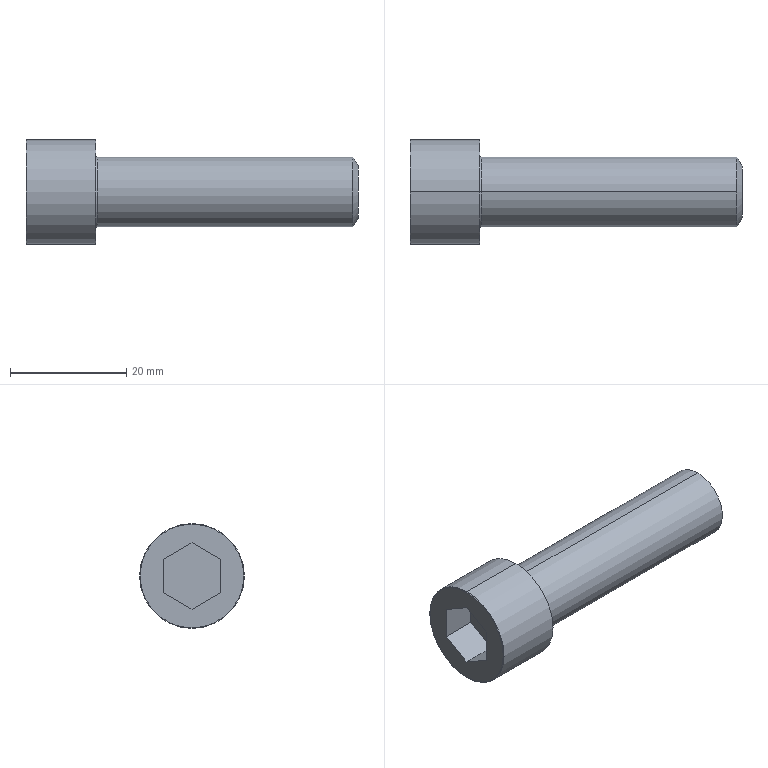Part | SolidWorks | features BlendCut 1, Cut 1, Fillet 1, LPattern 1, RevCut 1, Revolution 1 | 1 solid | 20 faces | box 57 x 18 x 18 mm | volume 7611 mm3 | plane 10 | torus 4 | cylinder 4 | cone 2 | commonest cylinder face diameters 12 x2 18 x2
STEP:
#1=CARTESIAN_POINT('',(0.,0.,8.9));
#2=VERTEX_POINT('',#1);
#3=CARTESIAN_POINT('',(0.,0.,-8.9));
#4=VERTEX_POINT('',#3);
#5=CARTESIAN_POINT('',(0.,0.,0.));
#6=DIRECTION('',(-1.,0.,0.));
#7=DIRECTION('',(0.,0.,-1.));
#8=AXIS2_PLACEMENT_3D('',#5,#6,#7);
#9=CIRCLE('',#8,8.9);
#10=EDGE_CURVE('',#2,#4,#9,.T.);
#11=ORIENTED_EDGE('',*,*,#10,.F.);
#12=CARTESIAN_POINT('',(0.1,0.,9.));
#13=VERTEX_POINT('',#12);
#14=CARTESIAN_POINT('',(0.1,0.,8.9));
#15=DIRECTION('',(0.,1.,0.));
#16=DIRECTION('',(0.,0.,1.));
#17=AXIS2_PLACEMENT_3D('',#14,#15,#16);
#18=CIRCLE('',#17,0.1);
#19=EDGE_CURVE('',#2,#13,#18,.T.);
#20=ORIENTED_EDGE('',*,*,#19,.T.);
#21=CARTESIAN_POINT('',(0.1,0.,-9.));
#22=VERTEX_POINT('',#21);
#23=CARTESIAN_POINT('',(0.1,0.,0.));
#24=DIRECTION('',(1.,0.,0.));
#25=DIRECTION('',(0.,0.,-1.));
#26=AXIS2_PLACEMENT_3D('',#23,#24,#25);
#27=CIRCLE('',#26,9.);
#28=EDGE_CURVE('',#22,#13,#27,.T.);
#29=ORIENTED_EDGE('',*,*,#28,.F.);
#30=CARTESIAN_POINT('',(0.1,0.,-8.9));
#31=DIRECTION('',(0.,-1.,0.));
#32=DIRECTION('',(0.,0.,-1.));
#33=AXIS2_PLACEMENT_3D('',#30,#31,#32);
#34=CIRCLE('',#33,0.1);
#35=EDGE_CURVE('',#4,#22,#34,.T.);
#36=ORIENTED_EDGE('',*,*,#35,.F.);
#37=EDGE_LOOP('',(#11,#20,#29,#36));
#38=FACE_OUTER_BOUND('',#37,.T.);
#39=CARTESIAN_POINT('',(0.1,0.,0.));
#40=DIRECTION('',(1.,0.,0.));
#41=DIRECTION('',(0.,0.,-1.));
#42=AXIS2_PLACEMENT_3D('',#39,#40,#41);
#43=TOROIDAL_SURFACE('',#42,8.9,0.1);
#44=ADVANCED_FACE('',(#38),#43,.T.);
#45=CARTESIAN_POINT('',(57.,0.,4.485));
#46=VERTEX_POINT('',#45);
#47=CARTESIAN_POINT('',(57.,0.,-4.485));
#48=VERTEX_POINT('',#47);
#49=CARTESIAN_POINT('',(57.,0.,0.));
#50=DIRECTION('',(-1.,0.,0.));
#51=DIRECTION('',(0.,0.,1.));
#52=AXIS2_PLACEMENT_3D('',#49,#50,#51);
#53=CIRCLE('',#52,4.485);
#54=EDGE_CURVE('',#46,#48,#53,.T.);
#55=ORIENTED_EDGE('',*,*,#54,.T.);
#56=CARTESIAN_POINT('',(56.125,0.,-6.));
#57=VERTEX_POINT('',#56);
#58=CARTESIAN_POINT('',(56.125,0.,-6.));
#59=DIRECTION('',(-0.5,0.,-0.866));
#60=VECTOR('',#59,1000.);
#61=LINE('',#58,#60);
#62=EDGE_CURVE('',#48,#57,#61,.T.);
#63=ORIENTED_EDGE('',*,*,#62,.T.);
#64=CARTESIAN_POINT('',(56.125,0.,6.));
#65=VERTEX_POINT('',#64);
#66=CARTESIAN_POINT('',(56.125,0.,0.));
#67=DIRECTION('',(-1.,0.,0.));
#68=DIRECTION('',(0.,0.,1.));
#69=AXIS2_PLACEMENT_3D('',#66,#67,#68);
#70=CIRCLE('',#69,6.);
#71=EDGE_CURVE('',#65,#57,#70,.T.);
#72=ORIENTED_EDGE('',*,*,#71,.F.);
#73=CARTESIAN_POINT('',(56.125,0.,6.));
#74=DIRECTION('',(-0.5,0.,0.866));
#75=VECTOR('',#74,1000.);
#76=LINE('',#73,#75);
#77=EDGE_CURVE('',#46,#65,#76,.T.);
#78=ORIENTED_EDGE('',*,*,#77,.F.);
#79=EDGE_LOOP('',(#55,#63,#72,#78));
#80=FACE_OUTER_BOUND('',#79,.T.);
#81=CARTESIAN_POINT('',(56.125,0.,0.));
#82=DIRECTION('',(-1.,0.,0.));
#83=DIRECTION('',(0.,0.,1.));
#84=AXIS2_PLACEMENT_3D('',#81,#82,#83);
#85=CONICAL_SURFACE('',#84,6.,1.047);
#86=ADVANCED_FACE('',(#80),#85,.T.);
#87=CARTESIAN_POINT('',(12.,0.,-6.2));
#88=VERTEX_POINT('',#87);
#89=CARTESIAN_POINT('',(12.,0.,6.2));
#90=VERTEX_POINT('',#89);
#91=CARTESIAN_POINT('',(12.,0.,0.));
#92=DIRECTION('',(-1.,0.,0.));
#93=DIRECTION('',(0.,0.,1.));
#94=AXIS2_PLACEMENT_3D('',#91,#92,#93);
#95=CIRCLE('',#94,6.2);
#96=EDGE_CURVE('',#88,#90,#95,.T.);
#97=ORIENTED_EDGE('',*,*,#96,.F.);
#98=CARTESIAN_POINT('',(12.2,0.,-6.));
#99=VERTEX_POINT('',#98);
#100=CARTESIAN_POINT('',(12.2,0.,-6.2));
#101=DIRECTION('',(0.,1.,0.));
#102=DIRECTION('',(0.,0.,1.));
#103=AXIS2_PLACEMENT_3D('',#100,#101,#102);
#104=CIRCLE('',#103,0.2);
#105=EDGE_CURVE('',#88,#99,#104,.T.);
#106=ORIENTED_EDGE('',*,*,#105,.T.);
#107=CARTESIAN_POINT('',(12.2,0.,6.));
#108=VERTEX_POINT('',#107);
#109=CARTESIAN_POINT('',(12.2,0.,0.));
#110=DIRECTION('',(-1.,0.,0.));
#111=DIRECTION('',(0.,0.,1.));
#112=AXIS2_PLACEMENT_3D('',#109,#110,#111);
#113=CIRCLE('',#112,6.);
#114=EDGE_CURVE('',#99,#108,#113,.T.);
#115=ORIENTED_EDGE('',*,*,#114,.T.);
#116=CARTESIAN_POINT('',(12.2,0.,6.2));
#117=DIRECTION('',(0.,-1.,0.));
#118=DIRECTION('',(0.,0.,-1.));
#119=AXIS2_PLACEMENT_3D('',#116,#117,#118);
#120=CIRCLE('',#119,0.2);
#121=EDGE_CURVE('',#90,#108,#120,.T.);
#122=ORIENTED_EDGE('',*,*,#121,.F.);
#123=EDGE_LOOP('',(#97,#106,#115,#122));
#124=FACE_OUTER_BOUND('',#123,.T.);
#125=CARTESIAN_POINT('',(12.2,0.,0.));
#126=DIRECTION('',(-1.,0.,0.));
#127=DIRECTION('',(0.,0.,1.));
#128=AXIS2_PLACEMENT_3D('',#125,#126,#127);
#129=TOROIDAL_SURFACE('',#128,6.2,0.2);
#130=ADVANCED_FACE('',(#124),#129,.F.);
#131=CARTESIAN_POINT('',(12.,0.,9.));
#132=VERTEX_POINT('',#131);
#133=CARTESIAN_POINT('',(12.,0.,-9.));
#134=VERTEX_POINT('',#133);
#135=CARTESIAN_POINT('',(12.,0.,0.));
#136=DIRECTION('',(-1.,0.,0.));
#137=DIRECTION('',(0.,0.,1.));
#138=AXIS2_PLACEMENT_3D('',#135,#136,#137);
#139=CIRCLE('',#138,9.);
#140=EDGE_CURVE('',#132,#134,#139,.T.);
#141=ORIENTED_EDGE('',*,*,#140,.T.);
#142=CARTESIAN_POINT('',(0.,0.,-9.));
#143=DIRECTION('',(-1.,0.,0.));
#144=VECTOR('',#143,1000.);
#145=LINE('',#142,#144);
#146=EDGE_CURVE('',#134,#22,#145,.T.);
#147=ORIENTED_EDGE('',*,*,#146,.T.);
#148=ORIENTED_EDGE('',*,*,#28,.T.);
#149=CARTESIAN_POINT('',(0.,0.,9.));
#150=DIRECTION('',(-1.,0.,0.));
#151=VECTOR('',#150,1000.);
#152=LINE('',#149,#151);
#153=EDGE_CURVE('',#132,#13,#152,.T.);
#154=ORIENTED_EDGE('',*,*,#153,.F.);
#155=EDGE_LOOP('',(#141,#147,#148,#154));
#156=FACE_OUTER_BOUND('',#155,.T.);
#157=CARTESIAN_POINT('',(0.,0.,0.));
#158=DIRECTION('',(-1.,0.,0.));
#159=DIRECTION('',(0.,0.,1.));
#160=AXIS2_PLACEMENT_3D('',#157,#158,#159);
#161=CYLINDRICAL_SURFACE('',#160,9.);
#162=ADVANCED_FACE('',(#156),#161,.T.);
#163=ORIENTED_EDGE('',*,*,#71,.T.);
#164=CARTESIAN_POINT('',(0.,0.,-6.));
#165=DIRECTION('',(-1.,0.,0.));
#166=VECTOR('',#165,1000.);
#167=LINE('',#164,#166);
#168=EDGE_CURVE('',#57,#99,#167,.T.);
#169=ORIENTED_EDGE('',*,*,#168,.T.);
#170=CARTESIAN_POINT('',(12.2,0.,0.));
#171=DIRECTION('',(-1.,0.,0.));
#172=DIRECTION('',(0.,0.,1.));
#173=AXIS2_PLACEMENT_3D('',#170,#171,#172);
#174=CIRCLE('',#173,6.);
#175=EDGE_CURVE('',#108,#99,#174,.T.);
#176=ORIENTED_EDGE('',*,*,#175,.F.);
#177=CARTESIAN_POINT('',(0.,0.,6.));
#178=DIRECTION('',(-1.,0.,0.));
#179=VECTOR('',#178,1000.);
#180=LINE('',#177,#179);
#181=EDGE_CURVE('',#65,#108,#180,.T.);
#182=ORIENTED_EDGE('',*,*,#181,.F.);
#183=EDGE_LOOP('',(#163,#169,#176,#182));
#184=FACE_OUTER_BOUND('',#183,.T.);
#185=CARTESIAN_POINT('',(0.,0.,0.));
#186=DIRECTION('',(-1.,0.,0.));
#187=DIRECTION('',(0.,0.,1.));
#188=AXIS2_PLACEMENT_3D('',#185,#186,#187);
#189=CYLINDRICAL_SURFACE('',#188,6.);
#190=ADVANCED_FACE('',(#184),#189,.T.);
#191=ORIENTED_EDGE('',*,*,#168,.F.);
#192=CARTESIAN_POINT('',(56.125,0.,0.));
#193=DIRECTION('',(-1.,0.,0.));
#194=DIRECTION('',(0.,0.,1.));
#195=AXIS2_PLACEMENT_3D('',#192,#193,#194);
#196=CIRCLE('',#195,6.);
#197=EDGE_CURVE('',#57,#65,#196,.T.);
#198=ORIENTED_EDGE('',*,*,#197,.T.);
#199=ORIENTED_EDGE('',*,*,#181,.T.);
#200=ORIENTED_EDGE('',*,*,#114,.F.);
#201=EDGE_LOOP('',(#191,#198,#199,#200));
#202=FACE_OUTER_BOUND('',#201,.T.);
#203=CARTESIAN_POINT('',(0.,0.,0.));
#204=DIRECTION('',(-1.,0.,0.));
#205=DIRECTION('',(0.,0.,1.));
#206=AXIS2_PLACEMENT_3D('',#203,#204,#205);
#207=CYLINDRICAL_SURFACE('',#206,6.);
#208=ADVANCED_FACE('',(#202),#207,.T.);
#209=CARTESIAN_POINT('',(0.,0.,0.));
#210=DIRECTION('',(-1.,0.,0.));
#211=DIRECTION('',(0.,0.,-1.));
#212=AXIS2_PLACEMENT_3D('',#209,#210,#211);
#213=CIRCLE('',#212,8.9);
#214=EDGE_CURVE('',#4,#2,#213,.T.);
#215=ORIENTED_EDGE('',*,*,#214,.T.);
#216=ORIENTED_EDGE('',*,*,#10,.T.);
#217=EDGE_LOOP('',(#215,#216));
#218=FACE_OUTER_BOUND('',#217,.T.);
#219=CARTESIAN_POINT('',(0.,0.,5.715));
#220=VERTEX_POINT('',#219);
#221=CARTESIAN_POINT('',(0.,4.949,2.857));
#222=VERTEX_POINT('',#221);
#223=CARTESIAN_POINT('',(0.,0.,5.715));
#224=DIRECTION('',(0.,0.866,-0.5));
#225=VECTOR('',#224,1000.);
#226=LINE('',#223,#225);
#227=EDGE_CURVE('',#220,#222,#226,.T.);
#228=ORIENTED_EDGE('',*,*,#227,.F.);
#229=CARTESIAN_POINT('',(0.,-4.949,2.858));
#230=VERTEX_POINT('',#229);
#231=CARTESIAN_POINT('',(0.,-4.949,2.858));
#232=DIRECTION('',(0.,0.866,0.5));
#233=VECTOR('',#232,1000.);
#234=LINE('',#231,#233);
#235=EDGE_CURVE('',#230,#220,#234,.T.);
#236=ORIENTED_EDGE('',*,*,#235,.F.);
#237=CARTESIAN_POINT('',(0.,-4.949,-2.857));
#238=VERTEX_POINT('',#237);
#239=CARTESIAN_POINT('',(0.,-4.949,-2.857));
#240=DIRECTION('',(0.,0.,1.));
#241=VECTOR('',#240,1000.);
#242=LINE('',#239,#241);
#243=EDGE_CURVE('',#238,#230,#242,.T.);
#244=ORIENTED_EDGE('',*,*,#243,.F.);
#245=CARTESIAN_POINT('',(0.,0.,-5.715));
#246=VERTEX_POINT('',#245);
#247=CARTESIAN_POINT('',(0.,0.,-5.715));
#248=DIRECTION('',(0.,-0.866,0.5));
#249=VECTOR('',#248,1000.);
#250=LINE('',#247,#249);
#251=EDGE_CURVE('',#246,#238,#250,.T.);
#252=ORIENTED_EDGE('',*,*,#251,.F.);
#253=CARTESIAN_POINT('',(0.,4.949,-2.857));
#254=VERTEX_POINT('',#253);
#255=CARTESIAN_POINT('',(0.,4.949,-2.857));
#256=DIRECTION('',(0.,-0.866,-0.5));
#257=VECTOR('',#256,1000.);
#258=LINE('',#255,#257);
#259=EDGE_CURVE('',#254,#246,#258,.T.);
#260=ORIENTED_EDGE('',*,*,#259,.F.);
#261=CARTESIAN_POINT('',(0.,4.949,2.857));
#262=DIRECTION('',(0.,0.,-1.));
#263=VECTOR('',#262,1000.);
#264=LINE('',#261,#263);
#265=EDGE_CURVE('',#222,#254,#264,.T.);
#266=ORIENTED_EDGE('',*,*,#265,.F.);
#267=EDGE_LOOP('',(#228,#236,#244,#252,#260,#266));
#268=FACE_BOUND('',#267,.T.);
#269=CARTESIAN_POINT('',(0.,0.,0.));
#270=DIRECTION('',(1.,0.,0.));
#271=DIRECTION('',(0.,0.,-1.));
#272=AXIS2_PLACEMENT_3D('',#269,#270,#271);
#273=PLANE('',#272);
#274=ADVANCED_FACE('',(#218,#268),#273,.F.);
#275=ORIENTED_EDGE('',*,*,#146,.F.);
#276=CARTESIAN_POINT('',(12.,0.,0.));
#277=DIRECTION('',(-1.,0.,0.));
#278=DIRECTION('',(0.,0.,1.));
#279=AXIS2_PLACEMENT_3D('',#276,#277,#278);
#280=CIRCLE('',#279,9.);
#281=EDGE_CURVE('',#134,#132,#280,.T.);
#282=ORIENTED_EDGE('',*,*,#281,.T.);
#283=ORIENTED_EDGE('',*,*,#153,.T.);
#284=CARTESIAN_POINT('',(0.1,0.,0.));
#285=DIRECTION('',(1.,0.,0.));
#286=DIRECTION('',(0.,0.,-1.));
#287=AXIS2_PLACEMENT_3D('',#284,#285,#286);
#288=CIRCLE('',#287,9.);
#289=EDGE_CURVE('',#13,#22,#288,.T.);
#290=ORIENTED_EDGE('',*,*,#289,.T.);
#291=EDGE_LOOP('',(#275,#282,#283,#290));
#292=FACE_OUTER_BOUND('',#291,.T.);
#293=CARTESIAN_POINT('',(0.,0.,0.));
#294=DIRECTION('',(-1.,0.,0.));
#295=DIRECTION('',(0.,0.,1.));
#296=AXIS2_PLACEMENT_3D('',#293,#294,#295);
#297=CYLINDRICAL_SURFACE('',#296,9.);
#298=ADVANCED_FACE('',(#292),#297,.T.);
#299=ORIENTED_EDGE('',*,*,#140,.F.);
#300=ORIENTED_EDGE('',*,*,#281,.F.);
#301=EDGE_LOOP('',(#299,#300));
#302=FACE_OUTER_BOUND('',#301,.T.);
#303=CARTESIAN_POINT('',(12.,0.,0.));
#304=DIRECTION('',(-1.,0.,0.));
#305=DIRECTION('',(0.,0.,1.));
#306=AXIS2_PLACEMENT_3D('',#303,#304,#305);
#307=CIRCLE('',#306,6.2);
#308=EDGE_CURVE('',#90,#88,#307,.T.);
#309=ORIENTED_EDGE('',*,*,#308,.T.);
#310=ORIENTED_EDGE('',*,*,#96,.T.);
#311=EDGE_LOOP('',(#309,#310));
#312=FACE_BOUND('',#311,.T.);
#313=CARTESIAN_POINT('',(12.,9.,0.));
#314=DIRECTION('',(-1.,0.,0.));
#315=DIRECTION('',(0.,0.,1.));
#316=AXIS2_PLACEMENT_3D('',#313,#314,#315);
#317=PLANE('',#316);
#318=ADVANCED_FACE('',(#302,#312),#317,.F.);
#319=ORIENTED_EDGE('',*,*,#105,.F.);
#320=ORIENTED_EDGE('',*,*,#308,.F.);
#321=ORIENTED_EDGE('',*,*,#121,.T.);
#322=ORIENTED_EDGE('',*,*,#175,.T.);
#323=EDGE_LOOP('',(#319,#320,#321,#322));
#324=FACE_OUTER_BOUND('',#323,.T.);
#325=CARTESIAN_POINT('',(12.2,0.,0.));
#326=DIRECTION('',(-1.,0.,0.));
#327=DIRECTION('',(0.,0.,1.));
#328=AXIS2_PLACEMENT_3D('',#325,#326,#327);
#329=TOROIDAL_SURFACE('',#328,6.2,0.2);
#330=ADVANCED_FACE('',(#324),#329,.F.);
#331=ORIENTED_EDGE('',*,*,#235,.T.);
#332=CARTESIAN_POINT('',(6.,0.,5.715));
#333=VERTEX_POINT('',#332);
#334=CARTESIAN_POINT('',(6.,0.,5.715));
#335=DIRECTION('',(-1.,0.,0.));
#336=VECTOR('',#335,1000.);
#337=LINE('',#334,#336);
#338=EDGE_CURVE('',#333,#220,#337,.T.);
#339=ORIENTED_EDGE('',*,*,#338,.F.);
#340=CARTESIAN_POINT('',(6.,-4.949,2.858));
#341=VERTEX_POINT('',#340);
#342=CARTESIAN_POINT('',(6.,-4.949,2.858));
#343=DIRECTION('',(0.,0.866,0.5));
#344=VECTOR('',#343,1000.);
#345=LINE('',#342,#344);
#346=EDGE_CURVE('',#341,#333,#345,.T.);
#347=ORIENTED_EDGE('',*,*,#346,.F.);
#348=CARTESIAN_POINT('',(6.,-4.949,2.858));
#349=DIRECTION('',(-1.,0.,0.));
#350=VECTOR('',#349,1000.);
#351=LINE('',#348,#350);
#352=EDGE_CURVE('',#341,#230,#351,.T.);
#353=ORIENTED_EDGE('',*,*,#352,.T.);
#354=EDGE_LOOP('',(#331,#339,#347,#353));
#355=FACE_OUTER_BOUND('',#354,.T.);
#356=CARTESIAN_POINT('',(6.,-4.949,2.858));
#357=DIRECTION('',(0.,-0.5,0.866));
#358=DIRECTION('',(0.,-0.866,-0.5));
#359=AXIS2_PLACEMENT_3D('',#356,#357,#358);
#360=PLANE('',#359);
#361=ADVANCED_FACE('',(#355),#360,.F.);
#362=ORIENTED_EDGE('',*,*,#243,.T.);
#363=ORIENTED_EDGE('',*,*,#352,.F.);
#364=CARTESIAN_POINT('',(6.,-4.949,-2.857));
#365=VERTEX_POINT('',#364);
#366=CARTESIAN_POINT('',(6.,-4.949,-2.857));
#367=DIRECTION('',(0.,0.,1.));
#368=VECTOR('',#367,1000.);
#369=LINE('',#366,#368);
#370=EDGE_CURVE('',#365,#341,#369,.T.);
#371=ORIENTED_EDGE('',*,*,#370,.F.);
#372=CARTESIAN_POINT('',(6.,-4.949,-2.857));
#373=DIRECTION('',(-1.,0.,0.));
#374=VECTOR('',#373,1000.);
#375=LINE('',#372,#374);
#376=EDGE_CURVE('',#365,#238,#375,.T.);
#377=ORIENTED_EDGE('',*,*,#376,.T.);
#378=EDGE_LOOP('',(#362,#363,#371,#377));
#379=FACE_OUTER_BOUND('',#378,.T.);
#380=CARTESIAN_POINT('',(6.,-4.949,-2.857));
#381=DIRECTION('',(0.,-1.,0.));
#382=DIRECTION('',(0.,0.,-1.));
#383=AXIS2_PLACEMENT_3D('',#380,#381,#382);
#384=PLANE('',#383);
#385=ADVANCED_FACE('',(#379),#384,.F.);
#386=ORIENTED_EDGE('',*,*,#251,.T.);
#387=ORIENTED_EDGE('',*,*,#376,.F.);
#388=CARTESIAN_POINT('',(6.,0.,-5.715));
#389=VERTEX_POINT('',#388);
#390=CARTESIAN_POINT('',(6.,0.,-5.715));
#391=DIRECTION('',(0.,-0.866,0.5));
#392=VECTOR('',#391,1000.);
#393=LINE('',#390,#392);
#394=EDGE_CURVE('',#389,#365,#393,.T.);
#395=ORIENTED_EDGE('',*,*,#394,.F.);
#396=CARTESIAN_POINT('',(6.,0.,-5.715));
#397=DIRECTION('',(-1.,0.,0.));
#398=VECTOR('',#397,1000.);
#399=LINE('',#396,#398);
#400=EDGE_CURVE('',#389,#246,#399,.T.);
#401=ORIENTED_EDGE('',*,*,#400,.T.);
#402=EDGE_LOOP('',(#386,#387,#395,#401));
#403=FACE_OUTER_BOUND('',#402,.T.);
#404=CARTESIAN_POINT('',(6.,0.,-5.715));
#405=DIRECTION('',(0.,-0.5,-0.866));
#406=DIRECTION('',(0.,0.866,-0.5));
#407=AXIS2_PLACEMENT_3D('',#404,#405,#406);
#408=PLANE('',#407);
#409=ADVANCED_FACE('',(#403),#408,.F.);
#410=ORIENTED_EDGE('',*,*,#259,.T.);
#411=ORIENTED_EDGE('',*,*,#400,.F.);
#412=CARTESIAN_POINT('',(6.,4.949,-2.857));
#413=VERTEX_POINT('',#412);
#414=CARTESIAN_POINT('',(6.,4.949,-2.857));
#415=DIRECTION('',(0.,-0.866,-0.5));
#416=VECTOR('',#415,1000.);
#417=LINE('',#414,#416);
#418=EDGE_CURVE('',#413,#389,#417,.T.);
#419=ORIENTED_EDGE('',*,*,#418,.F.);
#420=CARTESIAN_POINT('',(6.,4.949,-2.857));
#421=DIRECTION('',(-1.,0.,0.));
#422=VECTOR('',#421,1000.);
#423=LINE('',#420,#422);
#424=EDGE_CURVE('',#413,#254,#423,.T.);
#425=ORIENTED_EDGE('',*,*,#424,.T.);
#426=EDGE_LOOP('',(#410,#411,#419,#425));
#427=FACE_OUTER_BOUND('',#426,.T.);
#428=CARTESIAN_POINT('',(6.,4.949,-2.857));
#429=DIRECTION('',(0.,0.5,-0.866));
#430=DIRECTION('',(0.,0.866,0.5));
#431=AXIS2_PLACEMENT_3D('',#428,#429,#430);
#432=PLANE('',#431);
#433=ADVANCED_FACE('',(#427),#432,.F.);
#434=ORIENTED_EDGE('',*,*,#265,.T.);
#435=ORIENTED_EDGE('',*,*,#424,.F.);
#436=CARTESIAN_POINT('',(6.,4.949,2.857));
#437=VERTEX_POINT('',#436);
#438=CARTESIAN_POINT('',(6.,4.949,2.857));
#439=DIRECTION('',(0.,0.,-1.));
#440=VECTOR('',#439,1000.);
#441=LINE('',#438,#440);
#442=EDGE_CURVE('',#437,#413,#441,.T.);
#443=ORIENTED_EDGE('',*,*,#442,.F.);
#444=CARTESIAN_POINT('',(6.,4.949,2.857));
#445=DIRECTION('',(-1.,0.,0.));
#446=VECTOR('',#445,1000.);
#447=LINE('',#444,#446);
#448=EDGE_CURVE('',#437,#222,#447,.T.);
#449=ORIENTED_EDGE('',*,*,#448,.T.);
#450=EDGE_LOOP('',(#434,#435,#443,#449));
#451=FACE_OUTER_BOUND('',#450,.T.);
#452=CARTESIAN_POINT('',(6.,4.949,2.857));
#453=DIRECTION('',(0.,1.,0.));
#454=DIRECTION('',(0.,0.,1.));
#455=AXIS2_PLACEMENT_3D('',#452,#453,#454);
#456=PLANE('',#455);
#457=ADVANCED_FACE('',(#451),#456,.F.);
#458=ORIENTED_EDGE('',*,*,#227,.T.);
#459=ORIENTED_EDGE('',*,*,#448,.F.);
#460=CARTESIAN_POINT('',(6.,0.,5.715));
#461=DIRECTION('',(0.,0.866,-0.5));
#462=VECTOR('',#461,1000.);
#463=LINE('',#460,#462);
#464=EDGE_CURVE('',#333,#437,#463,.T.);
#465=ORIENTED_EDGE('',*,*,#464,.F.);
#466=ORIENTED_EDGE('',*,*,#338,.T.);
#467=EDGE_LOOP('',(#458,#459,#465,#466));
#468=FACE_OUTER_BOUND('',#467,.T.);
#469=CARTESIAN_POINT('',(6.,0.,5.715));
#470=DIRECTION('',(0.,0.5,0.866));
#471=DIRECTION('',(0.,-0.866,0.5));
#472=AXIS2_PLACEMENT_3D('',#469,#470,#471);
#473=PLANE('',#472);
#474=ADVANCED_FACE('',(#468),#473,.F.);
#475=ORIENTED_EDGE('',*,*,#346,.T.);
#476=ORIENTED_EDGE('',*,*,#464,.T.);
#477=ORIENTED_EDGE('',*,*,#442,.T.);
#478=ORIENTED_EDGE('',*,*,#418,.T.);
#479=ORIENTED_EDGE('',*,*,#394,.T.);
#480=ORIENTED_EDGE('',*,*,#370,.T.);
#481=EDGE_LOOP('',(#475,#476,#477,#478,#479,#480));
#482=FACE_OUTER_BOUND('',#481,.T.);
#483=CARTESIAN_POINT('',(6.,-4.949,2.858));
#484=DIRECTION('',(1.,0.,0.));
#485=DIRECTION('',(0.,0.,-1.));
#486=AXIS2_PLACEMENT_3D('',#483,#484,#485);
#487=PLANE('',#486);
#488=ADVANCED_FACE('',(#482),#487,.F.);
#489=ORIENTED_EDGE('',*,*,#62,.F.);
#490=CARTESIAN_POINT('',(57.,0.,0.));
#491=DIRECTION('',(-1.,0.,0.));
#492=DIRECTION('',(0.,0.,1.));
#493=AXIS2_PLACEMENT_3D('',#490,#491,#492);
#494=CIRCLE('',#493,4.485);
#495=EDGE_CURVE('',#48,#46,#494,.T.);
#496=ORIENTED_EDGE('',*,*,#495,.T.);
#497=ORIENTED_EDGE('',*,*,#77,.T.);
#498=ORIENTED_EDGE('',*,*,#197,.F.);
#499=EDGE_LOOP('',(#489,#496,#497,#498));
#500=FACE_OUTER_BOUND('',#499,.T.);
#501=CARTESIAN_POINT('',(56.125,0.,0.));
#502=DIRECTION('',(-1.,0.,0.));
#503=DIRECTION('',(0.,0.,1.));
#504=AXIS2_PLACEMENT_3D('',#501,#502,#503);
#505=CONICAL_SURFACE('',#504,6.,1.047);
#506=ADVANCED_FACE('',(#500),#505,.T.);
#507=ORIENTED_EDGE('',*,*,#54,.F.);
#508=ORIENTED_EDGE('',*,*,#495,.F.);
#509=EDGE_LOOP('',(#507,#508));
#510=FACE_OUTER_BOUND('',#509,.T.);
#511=CARTESIAN_POINT('',(57.,6.,0.));
#512=DIRECTION('',(-1.,0.,0.));
#513=DIRECTION('',(0.,0.,1.));
#514=AXIS2_PLACEMENT_3D('',#511,#512,#513);
#515=PLANE('',#514);
#516=ADVANCED_FACE('',(#510),#515,.F.);
#517=ORIENTED_EDGE('',*,*,#19,.F.);
#518=ORIENTED_EDGE('',*,*,#214,.F.);
#519=ORIENTED_EDGE('',*,*,#35,.T.);
#520=ORIENTED_EDGE('',*,*,#289,.F.);
#521=EDGE_LOOP('',(#517,#518,#519,#520));
#522=FACE_OUTER_BOUND('',#521,.T.);
#523=CARTESIAN_POINT('',(0.1,0.,0.));
#524=DIRECTION('',(1.,0.,0.));
#525=DIRECTION('',(0.,0.,-1.));
#526=AXIS2_PLACEMENT_3D('',#523,#524,#525);
#527=TOROIDAL_SURFACE('',#526,8.9,0.1);
#528=ADVANCED_FACE('',(#522),#527,.T.);
#529=CLOSED_SHELL('',(#44,#86,#130,#162,#190,#208,#274,#298,#318,#330,#361,#385,#409,#433,#457,#474,#488,#506,#516,#528));
#530=MANIFOLD_SOLID_BREP('',#529);
#531=CARTESIAN_POINT('',(0.,0.,0.));
#532=DIRECTION('',(0.,0.,1.));
#533=DIRECTION('',(1.,0.,0.));
#534=AXIS2_PLACEMENT_3D('',#531,#532,#533);
#535=(LENGTH_UNIT()NAMED_UNIT(*)SI_UNIT(.MILLI.,.METRE.));
#536=UNCERTAINTY_MEASURE_WITH_UNIT(LENGTH_MEASURE(0.00001),#535,'','');
#537=(NAMED_UNIT(*)PLANE_ANGLE_UNIT()SI_UNIT($,.RADIAN.));
#538=(NAMED_UNIT(*)SI_UNIT($,.STERADIAN.)SOLID_ANGLE_UNIT());
#539=(GEOMETRIC_REPRESENTATION_CONTEXT(3)GLOBAL_UNCERTAINTY_ASSIGNED_CONTEXT((#536))GLOBAL_UNIT_ASSIGNED_CONTEXT((#535,#537,#538))REPRESENTATION_CONTEXT('',''));
#540=ADVANCED_BREP_SHAPE_REPRESENTATION('',(#530,#534),#539);